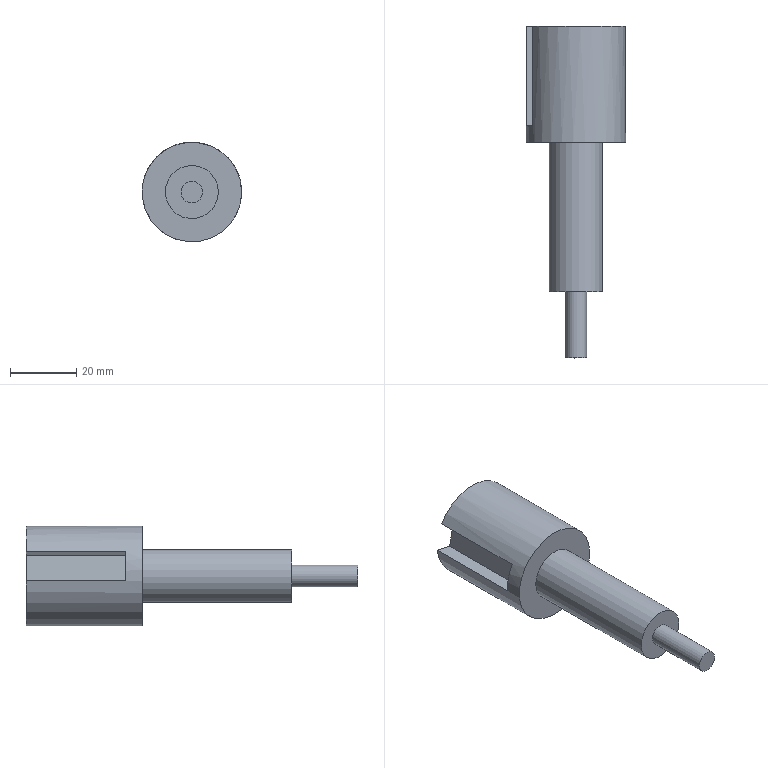Part | STEP file | SN10_006_001_PILOTO | 1 solid | 17 faces | box 30 x 100 x 30 mm | volume 30633 mm3 | plane 12 | cylinder 4 | cone 1 | commonest cylinder face diameters 6.5 x1 6.917 x1 16 x1 30 x1
STEP:
#1=CARTESIAN_POINT('',(0.,0.,0.));
#2=DIRECTION('',(0.,0.,1.));
#3=DIRECTION('',(1.,0.,0.));
#4=AXIS2_PLACEMENT_3D('',#1,#2,#3);
#5=CARTESIAN_POINT('',(381.092,-494.15,330.576));
#6=VERTEX_POINT('',#5);
#7=CARTESIAN_POINT('',(378.057,-494.15,328.918));
#8=DIRECTION('',(0.,1.,0.));
#9=DIRECTION('',(1.,0.,0.));
#10=AXIS2_PLACEMENT_3D('',#7,#8,#9);
#11=CIRCLE('',#10,3.458);
#12=CARTESIAN_POINT('',(378.057,-495.569,328.918));
#13=DIRECTION('',(0.,1.,0.));
#14=DIRECTION('',(0.8776,0.,0.4794));
#15=AXIS2_PLACEMENT_3D('',#12,#13,#14);
#16=CONICAL_SURFACE('',#15,1.,1.047);
#17=CARTESIAN_POINT('',(-5.783,1.419));
#18=DIRECTION('',(1.,0.));
#19=VECTOR('',#18,1.);
#20=LINE('',#17,#19);
#21=(GEOMETRIC_REPRESENTATION_CONTEXT(2)PARAMETRIC_REPRESENTATION_CONTEXT()REPRESENTATION_CONTEXT('',''));
#22=DEFINITIONAL_REPRESENTATION('',(#20),#21);
#23=PCURVE('',#16,#22);
#24=CARTESIAN_POINT('',(378.057,-476.25,328.918));
#25=DIRECTION('',(0.,-1.,0.));
#26=DIRECTION('',(0.8776,0.,0.4794));
#27=AXIS2_PLACEMENT_3D('',#24,#25,#26);
#28=CYLINDRICAL_SURFACE('',#27,3.458);
#29=CARTESIAN_POINT('',(12.066,17.9));
#30=DIRECTION('',(-1.,0.));
#31=VECTOR('',#30,1.);
#32=LINE('',#29,#31);
#33=(GEOMETRIC_REPRESENTATION_CONTEXT(2)PARAMETRIC_REPRESENTATION_CONTEXT()REPRESENTATION_CONTEXT('',''));
#34=DEFINITIONAL_REPRESENTATION('',(#32),#33);
#35=PCURVE('',#28,#34);
#36=SURFACE_CURVE('',#11,(#23,#35),.PCURVE_S1.);
#37=EDGE_CURVE('',#6,#6,#36,.T.);
#38=ORIENTED_EDGE('',*,*,#37,.F.);
#39=CARTESIAN_POINT('',(378.057,-496.147,328.918));
#40=VERTEX_POINT('',#39);
#41=CARTESIAN_POINT('',(378.057,-496.147,328.918));
#42=CARTESIAN_POINT('',(381.092,-494.15,330.576));
#43=B_SPLINE_CURVE_WITH_KNOTS('',1,(#41,#42),.UNSPECIFIED.,.F.,.F.,(2,2),(-1.155,2.839),.PIECEWISE_BEZIER_KNOTS.);
#44=CARTESIAN_POINT('',(0.,0.));
#45=DIRECTION('',(0.,1.));
#46=VECTOR('',#45,1.);
#47=LINE('',#44,#46);
#48=(GEOMETRIC_REPRESENTATION_CONTEXT(2)PARAMETRIC_REPRESENTATION_CONTEXT()REPRESENTATION_CONTEXT('',''));
#49=DEFINITIONAL_REPRESENTATION('',(#47),#48);
#50=PCURVE('',#16,#49);
#51=CARTESIAN_POINT('',(6.283,0.));
#52=DIRECTION('',(0.,1.));
#53=VECTOR('',#52,1.);
#54=LINE('',#51,#53);
#55=(GEOMETRIC_REPRESENTATION_CONTEXT(2)PARAMETRIC_REPRESENTATION_CONTEXT()REPRESENTATION_CONTEXT('',''));
#56=DEFINITIONAL_REPRESENTATION('',(#54),#55);
#57=PCURVE('',#16,#56);
#58=SEAM_CURVE('',#43,(#50,#57),.PCURVE_S1.);
#59=EDGE_CURVE('',#40,#6,#58,.T.);
#60=ORIENTED_EDGE('',*,*,#59,.F.);
#61=ORIENTED_EDGE('',*,*,#59,.T.);
#62=EDGE_LOOP('',(#38,#60,#61));
#63=FACE_BOUND('',#62,.F.);
#64=ADVANCED_FACE('',(#63),#16,.F.);
#65=CARTESIAN_POINT('',(391.135,-476.15,321.571));
#66=VERTEX_POINT('',#65);
#67=CARTESIAN_POINT('',(389.46,-476.15,319.173));
#68=VERTEX_POINT('',#67);
#69=CARTESIAN_POINT('',(378.057,-476.15,328.918));
#70=DIRECTION('',(0.,1.,0.));
#71=DIRECTION('',(1.,0.,0.));
#72=AXIS2_PLACEMENT_3D('',#69,#70,#71);
#73=CIRCLE('',#72,15.);
#74=CARTESIAN_POINT('',(392.736,-476.15,325.833));
#75=DIRECTION('',(0.,1.,0.));
#76=DIRECTION('',(0.,0.,1.));
#77=AXIS2_PLACEMENT_3D('',#74,#75,#76);
#78=PLANE('',#77);
#79=CARTESIAN_POINT('',(3.085,-14.679));
#80=DIRECTION('',(0.,1.));
#81=AXIS2_PLACEMENT_2D('',#79,#80);
#82=CIRCLE('',#81,15.);
#83=(GEOMETRIC_REPRESENTATION_CONTEXT(2)PARAMETRIC_REPRESENTATION_CONTEXT()REPRESENTATION_CONTEXT('',''));
#84=DEFINITIONAL_REPRESENTATION('',(#82),#83);
#85=PCURVE('',#78,#84);
#86=CARTESIAN_POINT('',(378.057,-526.15,328.918));
#87=DIRECTION('',(0.,1.,0.));
#88=DIRECTION('',(0.7602,0.,-0.6496));
#89=AXIS2_PLACEMENT_3D('',#86,#87,#88);
#90=CYLINDRICAL_SURFACE('',#89,15.);
#91=CARTESIAN_POINT('',(5.576,50.));
#92=DIRECTION('',(1.,0.));
#93=VECTOR('',#92,1.);
#94=LINE('',#91,#93);
#95=(GEOMETRIC_REPRESENTATION_CONTEXT(2)PARAMETRIC_REPRESENTATION_CONTEXT()REPRESENTATION_CONTEXT('',''));
#96=DEFINITIONAL_REPRESENTATION('',(#94),#95);
#97=PCURVE('',#90,#96);
#98=SURFACE_CURVE('',#73,(#85,#97),.PCURVE_S1.);
#99=EDGE_CURVE('',#66,#68,#98,.T.);
#100=ORIENTED_EDGE('',*,*,#99,.T.);
#101=CARTESIAN_POINT('',(363.128,-476.15,327.457));
#102=VERTEX_POINT('',#101);
#103=CARTESIAN_POINT('',(378.057,-476.15,328.918));
#104=DIRECTION('',(0.,1.,0.));
#105=DIRECTION('',(1.,0.,0.));
#106=AXIS2_PLACEMENT_3D('',#103,#104,#105);
#107=CIRCLE('',#106,15.);
#108=CARTESIAN_POINT('',(3.085,-14.679));
#109=DIRECTION('',(0.,1.));
#110=AXIS2_PLACEMENT_2D('',#108,#109);
#111=CIRCLE('',#110,15.);
#112=(GEOMETRIC_REPRESENTATION_CONTEXT(2)PARAMETRIC_REPRESENTATION_CONTEXT()REPRESENTATION_CONTEXT('',''));
#113=DEFINITIONAL_REPRESENTATION('',(#111),#112);
#114=PCURVE('',#78,#113);
#115=CARTESIAN_POINT('',(-0.7071,50.));
#116=DIRECTION('',(1.,0.));
#117=VECTOR('',#116,1.);
#118=LINE('',#115,#117);
#119=(GEOMETRIC_REPRESENTATION_CONTEXT(2)PARAMETRIC_REPRESENTATION_CONTEXT()REPRESENTATION_CONTEXT('',''));
#120=DEFINITIONAL_REPRESENTATION('',(#118),#119);
#121=PCURVE('',#90,#120);
#122=SURFACE_CURVE('',#107,(#114,#121),.PCURVE_S1.);
#123=EDGE_CURVE('',#68,#102,#122,.T.);
#124=ORIENTED_EDGE('',*,*,#123,.T.);
#125=CARTESIAN_POINT('',(368.324,-476.15,326.365));
#126=VERTEX_POINT('',#125);
#127=CARTESIAN_POINT('',(363.128,-476.15,327.457));
#128=DIRECTION('',(0.9786,0.,-0.2056));
#129=VECTOR('',#128,1.);
#130=LINE('',#127,#129);
#131=CARTESIAN_POINT('',(1.623,-29.608));
#132=DIRECTION('',(-0.2056,0.9786));
#133=VECTOR('',#132,1.);
#134=LINE('',#131,#133);
#135=(GEOMETRIC_REPRESENTATION_CONTEXT(2)PARAMETRIC_REPRESENTATION_CONTEXT()REPRESENTATION_CONTEXT('',''));
#136=DEFINITIONAL_REPRESENTATION('',(#134),#135);
#137=PCURVE('',#78,#136);
#138=CARTESIAN_POINT('',(363.128,-476.15,327.457));
#139=DIRECTION('',(-0.2056,0.,-0.9786));
#140=DIRECTION('',(-0.9786,0.,0.2056));
#141=AXIS2_PLACEMENT_3D('',#138,#139,#140);
#142=PLANE('',#141);
#143=CARTESIAN_POINT('',(0.,0.));
#144=DIRECTION('',(-1.,0.));
#145=VECTOR('',#144,1.);
#146=LINE('',#143,#145);
#147=(GEOMETRIC_REPRESENTATION_CONTEXT(2)PARAMETRIC_REPRESENTATION_CONTEXT()REPRESENTATION_CONTEXT('',''));
#148=DEFINITIONAL_REPRESENTATION('',(#146),#147);
#149=PCURVE('',#142,#148);
#150=SURFACE_CURVE('',#130,(#137,#149),.PCURVE_S1.);
#151=EDGE_CURVE('',#102,#126,#150,.T.);
#152=ORIENTED_EDGE('',*,*,#151,.T.);
#153=CARTESIAN_POINT('',(370.175,-476.15,335.172));
#154=VERTEX_POINT('',#153);
#155=CARTESIAN_POINT('',(368.324,-476.15,326.365));
#156=DIRECTION('',(0.2056,0.,0.9786));
#157=VECTOR('',#156,1.);
#158=LINE('',#155,#157);
#159=CARTESIAN_POINT('',(0.5316,-24.412));
#160=DIRECTION('',(0.9786,0.2056));
#161=VECTOR('',#160,1.);
#162=LINE('',#159,#161);
#163=(GEOMETRIC_REPRESENTATION_CONTEXT(2)PARAMETRIC_REPRESENTATION_CONTEXT()REPRESENTATION_CONTEXT('',''));
#164=DEFINITIONAL_REPRESENTATION('',(#162),#163);
#165=PCURVE('',#78,#164);
#166=CARTESIAN_POINT('',(368.324,-476.15,326.365));
#167=DIRECTION('',(0.9786,0.,-0.2056));
#168=DIRECTION('',(-0.2056,0.,-0.9786));
#169=AXIS2_PLACEMENT_3D('',#166,#167,#168);
#170=PLANE('',#169);
#171=CARTESIAN_POINT('',(0.,0.));
#172=DIRECTION('',(-1.,0.));
#173=VECTOR('',#172,1.);
#174=LINE('',#171,#173);
#175=(GEOMETRIC_REPRESENTATION_CONTEXT(2)PARAMETRIC_REPRESENTATION_CONTEXT()REPRESENTATION_CONTEXT('',''));
#176=DEFINITIONAL_REPRESENTATION('',(#174),#175);
#177=PCURVE('',#170,#176);
#178=SURFACE_CURVE('',#158,(#165,#177),.PCURVE_S1.);
#179=EDGE_CURVE('',#126,#154,#178,.T.);
#180=ORIENTED_EDGE('',*,*,#179,.T.);
#181=CARTESIAN_POINT('',(364.979,-476.15,336.264));
#182=VERTEX_POINT('',#181);
#183=CARTESIAN_POINT('',(370.175,-476.15,335.172));
#184=DIRECTION('',(-0.9786,0.,0.2056));
#185=VECTOR('',#184,1.);
#186=LINE('',#183,#185);
#187=CARTESIAN_POINT('',(9.339,-22.562));
#188=DIRECTION('',(0.2056,-0.9786));
#189=VECTOR('',#188,1.);
#190=LINE('',#187,#189);
#191=(GEOMETRIC_REPRESENTATION_CONTEXT(2)PARAMETRIC_REPRESENTATION_CONTEXT()REPRESENTATION_CONTEXT('',''));
#192=DEFINITIONAL_REPRESENTATION('',(#190),#191);
#193=PCURVE('',#78,#192);
#194=CARTESIAN_POINT('',(370.175,-476.15,335.172));
#195=DIRECTION('',(0.2056,0.,0.9786));
#196=DIRECTION('',(0.9786,0.,-0.2056));
#197=AXIS2_PLACEMENT_3D('',#194,#195,#196);
#198=PLANE('',#197);
#199=CARTESIAN_POINT('',(0.000000001,0.));
#200=DIRECTION('',(-1.,0.));
#201=VECTOR('',#200,1.);
#202=LINE('',#199,#201);
#203=(GEOMETRIC_REPRESENTATION_CONTEXT(2)PARAMETRIC_REPRESENTATION_CONTEXT()REPRESENTATION_CONTEXT('',''));
#204=DEFINITIONAL_REPRESENTATION('',(#202),#203);
#205=PCURVE('',#198,#204);
#206=SURFACE_CURVE('',#186,(#193,#205),.PCURVE_S1.);
#207=EDGE_CURVE('',#154,#182,#206,.T.);
#208=ORIENTED_EDGE('',*,*,#207,.T.);
#209=CARTESIAN_POINT('',(392.985,-476.15,330.379));
#210=VERTEX_POINT('',#209);
#211=CARTESIAN_POINT('',(378.057,-476.15,328.918));
#212=DIRECTION('',(0.,1.,0.));
#213=DIRECTION('',(1.,0.,0.));
#214=AXIS2_PLACEMENT_3D('',#211,#212,#213);
#215=CIRCLE('',#214,15.);
#216=CARTESIAN_POINT('',(3.085,-14.679));
#217=DIRECTION('',(0.,1.));
#218=AXIS2_PLACEMENT_2D('',#216,#217);
#219=CIRCLE('',#218,15.);
#220=(GEOMETRIC_REPRESENTATION_CONTEXT(2)PARAMETRIC_REPRESENTATION_CONTEXT()REPRESENTATION_CONTEXT('',''));
#221=DEFINITIONAL_REPRESENTATION('',(#219),#220);
#222=PCURVE('',#78,#221);
#223=CARTESIAN_POINT('',(-0.7071,50.));
#224=DIRECTION('',(1.,0.));
#225=VECTOR('',#224,1.);
#226=LINE('',#223,#225);
#227=(GEOMETRIC_REPRESENTATION_CONTEXT(2)PARAMETRIC_REPRESENTATION_CONTEXT()REPRESENTATION_CONTEXT('',''));
#228=DEFINITIONAL_REPRESENTATION('',(#226),#227);
#229=PCURVE('',#90,#228);
#230=SURFACE_CURVE('',#215,(#222,#229),.PCURVE_S1.);
#231=EDGE_CURVE('',#182,#210,#230,.T.);
#232=ORIENTED_EDGE('',*,*,#231,.T.);
#233=CARTESIAN_POINT('',(387.79,-476.15,331.471));
#234=VERTEX_POINT('',#233);
#235=CARTESIAN_POINT('',(392.985,-476.15,330.379));
#236=DIRECTION('',(-0.9786,0.,0.2056));
#237=VECTOR('',#236,1.);
#238=LINE('',#235,#237);
#239=CARTESIAN_POINT('',(4.546,0.2492));
#240=DIRECTION('',(0.2056,-0.9786));
#241=VECTOR('',#240,1.);
#242=LINE('',#239,#241);
#243=(GEOMETRIC_REPRESENTATION_CONTEXT(2)PARAMETRIC_REPRESENTATION_CONTEXT()REPRESENTATION_CONTEXT('',''));
#244=DEFINITIONAL_REPRESENTATION('',(#242),#243);
#245=PCURVE('',#78,#244);
#246=CARTESIAN_POINT('',(370.175,-476.15,335.172));
#247=DIRECTION('',(0.2056,0.,0.9786));
#248=DIRECTION('',(0.9786,0.,-0.2056));
#249=AXIS2_PLACEMENT_3D('',#246,#247,#248);
#250=PLANE('',#249);
#251=CARTESIAN_POINT('',(23.309,0.));
#252=DIRECTION('',(-1.,0.));
#253=VECTOR('',#252,1.);
#254=LINE('',#251,#253);
#255=(GEOMETRIC_REPRESENTATION_CONTEXT(2)PARAMETRIC_REPRESENTATION_CONTEXT()REPRESENTATION_CONTEXT('',''));
#256=DEFINITIONAL_REPRESENTATION('',(#254),#255);
#257=PCURVE('',#250,#256);
#258=SURFACE_CURVE('',#238,(#245,#257),.PCURVE_S1.);
#259=EDGE_CURVE('',#210,#234,#258,.T.);
#260=ORIENTED_EDGE('',*,*,#259,.T.);
#261=CARTESIAN_POINT('',(385.939,-476.15,322.663));
#262=VERTEX_POINT('',#261);
#263=CARTESIAN_POINT('',(385.939,-476.15,322.663));
#264=DIRECTION('',(0.2056,0.,0.9786));
#265=VECTOR('',#264,1.);
#266=LINE('',#263,#265);
#267=CARTESIAN_POINT('',(-3.17,-6.797));
#268=DIRECTION('',(0.9786,0.2056));
#269=VECTOR('',#268,1.);
#270=LINE('',#267,#269);
#271=(GEOMETRIC_REPRESENTATION_CONTEXT(2)PARAMETRIC_REPRESENTATION_CONTEXT()REPRESENTATION_CONTEXT('',''));
#272=DEFINITIONAL_REPRESENTATION('',(#270),#271);
#273=PCURVE('',#78,#272);
#274=CARTESIAN_POINT('',(385.939,-476.15,322.663));
#275=DIRECTION('',(0.9786,0.,-0.2056));
#276=DIRECTION('',(-0.2056,0.,-0.9786));
#277=AXIS2_PLACEMENT_3D('',#274,#275,#276);
#278=PLANE('',#277);
#279=CARTESIAN_POINT('',(0.,0.));
#280=DIRECTION('',(-1.,0.));
#281=VECTOR('',#280,1.);
#282=LINE('',#279,#281);
#283=(GEOMETRIC_REPRESENTATION_CONTEXT(2)PARAMETRIC_REPRESENTATION_CONTEXT()REPRESENTATION_CONTEXT('',''));
#284=DEFINITIONAL_REPRESENTATION('',(#282),#283);
#285=PCURVE('',#278,#284);
#286=SURFACE_CURVE('',#266,(#273,#285),.PCURVE_S1.);
#287=EDGE_CURVE('',#262,#234,#286,.T.);
#288=ORIENTED_EDGE('',*,*,#287,.F.);
#289=CARTESIAN_POINT('',(385.939,-476.15,322.663));
#290=DIRECTION('',(0.9786,0.,-0.2056));
#291=VECTOR('',#290,1.);
#292=LINE('',#289,#291);
#293=CARTESIAN_POINT('',(-3.17,-6.797));
#294=DIRECTION('',(-0.2056,0.9786));
#295=VECTOR('',#294,1.);
#296=LINE('',#293,#295);
#297=(GEOMETRIC_REPRESENTATION_CONTEXT(2)PARAMETRIC_REPRESENTATION_CONTEXT()REPRESENTATION_CONTEXT('',''));
#298=DEFINITIONAL_REPRESENTATION('',(#296),#297);
#299=PCURVE('',#78,#298);
#300=CARTESIAN_POINT('',(363.128,-476.15,327.457));
#301=DIRECTION('',(-0.2056,0.,-0.9786));
#302=DIRECTION('',(-0.9786,0.,0.2056));
#303=AXIS2_PLACEMENT_3D('',#300,#301,#302);
#304=PLANE('',#303);
#305=CARTESIAN_POINT('',(-23.309,0.));
#306=DIRECTION('',(-1.,0.));
#307=VECTOR('',#306,1.);
#308=LINE('',#305,#307);
#309=(GEOMETRIC_REPRESENTATION_CONTEXT(2)PARAMETRIC_REPRESENTATION_CONTEXT()REPRESENTATION_CONTEXT('',''));
#310=DEFINITIONAL_REPRESENTATION('',(#308),#309);
#311=PCURVE('',#304,#310);
#312=SURFACE_CURVE('',#292,(#299,#311),.PCURVE_S1.);
#313=EDGE_CURVE('',#262,#66,#312,.T.);
#314=ORIENTED_EDGE('',*,*,#313,.T.);
#315=EDGE_LOOP('',(#100,#124,#152,#180,#208,#232,#260,#288,#314));
#316=FACE_BOUND('',#315,.T.);
#317=CARTESIAN_POINT('',(381.092,-476.15,330.576));
#318=VERTEX_POINT('',#317);
#319=CARTESIAN_POINT('',(378.057,-476.15,328.918));
#320=DIRECTION('',(0.,1.,0.));
#321=DIRECTION('',(1.,0.,0.));
#322=AXIS2_PLACEMENT_3D('',#319,#320,#321);
#323=CIRCLE('',#322,3.458);
#324=CARTESIAN_POINT('',(3.085,-14.679));
#325=DIRECTION('',(0.,1.));
#326=AXIS2_PLACEMENT_2D('',#324,#325);
#327=CIRCLE('',#326,3.458);
#328=(GEOMETRIC_REPRESENTATION_CONTEXT(2)PARAMETRIC_REPRESENTATION_CONTEXT()REPRESENTATION_CONTEXT('',''));
#329=DEFINITIONAL_REPRESENTATION('',(#327),#328);
#330=PCURVE('',#78,#329);
#331=CARTESIAN_POINT('',(12.066,-0.1));
#332=DIRECTION('',(-1.,0.));
#333=VECTOR('',#332,1.);
#334=LINE('',#331,#333);
#335=(GEOMETRIC_REPRESENTATION_CONTEXT(2)PARAMETRIC_REPRESENTATION_CONTEXT()REPRESENTATION_CONTEXT('',''));
#336=DEFINITIONAL_REPRESENTATION('',(#334),#335);
#337=PCURVE('',#28,#336);
#338=SURFACE_CURVE('',#323,(#330,#337),.PCURVE_S1.);
#339=EDGE_CURVE('',#318,#318,#338,.T.);
#340=ORIENTED_EDGE('',*,*,#339,.F.);
#341=EDGE_LOOP('',(#340));
#342=FACE_BOUND('',#341,.T.);
#343=ADVANCED_FACE('',(#316,#342),#78,.T.);
#344=ORIENTED_EDGE('',*,*,#123,.F.);
#345=CARTESIAN_POINT('',(389.46,-511.15,319.173));
#346=VERTEX_POINT('',#345);
#347=CARTESIAN_POINT('',(389.46,-511.15,319.173));
#348=CARTESIAN_POINT('',(389.46,-476.15,319.173));
#349=B_SPLINE_CURVE_WITH_KNOTS('',1,(#347,#348),.UNSPECIFIED.,.F.,.F.,(2,2),(15.,50.),.PIECEWISE_BEZIER_KNOTS.);
#350=CARTESIAN_POINT('',(0.,0.));
#351=DIRECTION('',(0.,1.));
#352=VECTOR('',#351,1.);
#353=LINE('',#350,#352);
#354=(GEOMETRIC_REPRESENTATION_CONTEXT(2)PARAMETRIC_REPRESENTATION_CONTEXT()REPRESENTATION_CONTEXT('',''));
#355=DEFINITIONAL_REPRESENTATION('',(#353),#354);
#356=PCURVE('',#90,#355);
#357=CARTESIAN_POINT('',(6.283,0.));
#358=DIRECTION('',(0.,1.));
#359=VECTOR('',#358,1.);
#360=LINE('',#357,#359);
#361=(GEOMETRIC_REPRESENTATION_CONTEXT(2)PARAMETRIC_REPRESENTATION_CONTEXT()REPRESENTATION_CONTEXT('',''));
#362=DEFINITIONAL_REPRESENTATION('',(#360),#361);
#363=PCURVE('',#90,#362);
#364=SEAM_CURVE('',#349,(#356,#363),.PCURVE_S1.);
#365=EDGE_CURVE('',#346,#68,#364,.T.);
#366=ORIENTED_EDGE('',*,*,#365,.F.);
#367=CARTESIAN_POINT('',(378.057,-511.15,328.918));
#368=DIRECTION('',(0.,1.,0.));
#369=DIRECTION('',(1.,0.,0.));
#370=AXIS2_PLACEMENT_3D('',#367,#368,#369);
#371=CIRCLE('',#370,15.);
#372=CARTESIAN_POINT('',(-0.7071,15.));
#373=DIRECTION('',(1.,0.));
#374=VECTOR('',#373,1.);
#375=LINE('',#372,#374);
#376=(GEOMETRIC_REPRESENTATION_CONTEXT(2)PARAMETRIC_REPRESENTATION_CONTEXT()REPRESENTATION_CONTEXT('',''));
#377=DEFINITIONAL_REPRESENTATION('',(#375),#376);
#378=PCURVE('',#90,#377);
#379=CARTESIAN_POINT('',(385.886,-511.15,327.273));
#380=DIRECTION('',(0.,1.,0.));
#381=DIRECTION('',(0.,0.,1.));
#382=AXIS2_PLACEMENT_3D('',#379,#380,#381);
#383=PLANE('',#382);
#384=CARTESIAN_POINT('',(1.645,-7.829));
#385=DIRECTION('',(0.,1.));
#386=AXIS2_PLACEMENT_2D('',#384,#385);
#387=CIRCLE('',#386,15.);
#388=(GEOMETRIC_REPRESENTATION_CONTEXT(2)PARAMETRIC_REPRESENTATION_CONTEXT()REPRESENTATION_CONTEXT('',''));
#389=DEFINITIONAL_REPRESENTATION('',(#387),#388);
#390=PCURVE('',#383,#389);
#391=SURFACE_CURVE('',#371,(#378,#390),.PCURVE_S1.);
#392=EDGE_CURVE('',#346,#346,#391,.T.);
#393=ORIENTED_EDGE('',*,*,#392,.T.);
#394=ORIENTED_EDGE('',*,*,#365,.T.);
#395=ORIENTED_EDGE('',*,*,#99,.F.);
#396=CARTESIAN_POINT('',(391.135,-506.15,321.571));
#397=VERTEX_POINT('',#396);
#398=CARTESIAN_POINT('',(391.135,-506.15,321.571));
#399=DIRECTION('',(0.,1.,0.));
#400=VECTOR('',#399,1.);
#401=LINE('',#398,#400);
#402=CARTESIAN_POINT('',(6.088,20.));
#403=DIRECTION('',(0.,1.));
#404=VECTOR('',#403,1.);
#405=LINE('',#402,#404);
#406=(GEOMETRIC_REPRESENTATION_CONTEXT(2)PARAMETRIC_REPRESENTATION_CONTEXT()REPRESENTATION_CONTEXT('',''));
#407=DEFINITIONAL_REPRESENTATION('',(#405),#406);
#408=PCURVE('',#90,#407);
#409=CARTESIAN_POINT('',(-28.618,-30.));
#410=DIRECTION('',(0.,1.));
#411=VECTOR('',#410,1.);
#412=LINE('',#409,#411);
#413=(GEOMETRIC_REPRESENTATION_CONTEXT(2)PARAMETRIC_REPRESENTATION_CONTEXT()REPRESENTATION_CONTEXT('',''));
#414=DEFINITIONAL_REPRESENTATION('',(#412),#413);
#415=PCURVE('',#304,#414);
#416=SURFACE_CURVE('',#401,(#408,#415),.PCURVE_S1.);
#417=EDGE_CURVE('',#397,#66,#416,.T.);
#418=ORIENTED_EDGE('',*,*,#417,.F.);
#419=CARTESIAN_POINT('',(392.985,-506.15,330.379));
#420=VERTEX_POINT('',#419);
#421=CARTESIAN_POINT('',(378.057,-506.15,328.918));
#422=DIRECTION('',(0.,1.,0.));
#423=DIRECTION('',(1.,0.,0.));
#424=AXIS2_PLACEMENT_3D('',#421,#422,#423);
#425=CIRCLE('',#424,15.);
#426=CARTESIAN_POINT('',(-0.7071,20.));
#427=DIRECTION('',(1.,0.));
#428=VECTOR('',#427,1.);
#429=LINE('',#426,#428);
#430=(GEOMETRIC_REPRESENTATION_CONTEXT(2)PARAMETRIC_REPRESENTATION_CONTEXT()REPRESENTATION_CONTEXT('',''));
#431=DEFINITIONAL_REPRESENTATION('',(#429),#430);
#432=PCURVE('',#90,#431);
#433=CARTESIAN_POINT('',(0.,-506.15,0.));
#434=DIRECTION('',(0.,1.,0.));
#435=DIRECTION('',(0.,0.,1.));
#436=AXIS2_PLACEMENT_3D('',#433,#434,#435);
#437=PLANE('',#436);
#438=CARTESIAN_POINT('',(328.918,378.057));
#439=DIRECTION('',(0.,1.));
#440=AXIS2_PLACEMENT_2D('',#438,#439);
#441=CIRCLE('',#440,15.);
#442=(GEOMETRIC_REPRESENTATION_CONTEXT(2)PARAMETRIC_REPRESENTATION_CONTEXT()REPRESENTATION_CONTEXT('',''));
#443=DEFINITIONAL_REPRESENTATION('',(#441),#442);
#444=PCURVE('',#437,#443);
#445=SURFACE_CURVE('',#425,(#432,#444),.PCURVE_S1.);
#446=EDGE_CURVE('',#420,#397,#445,.T.);
#447=ORIENTED_EDGE('',*,*,#446,.F.);
#448=CARTESIAN_POINT('',(392.985,-506.15,330.379));
#449=DIRECTION('',(0.,1.,0.));
#450=VECTOR('',#449,1.);
#451=LINE('',#448,#450);
#452=CARTESIAN_POINT('',(5.478,20.));
#453=DIRECTION('',(0.,1.));
#454=VECTOR('',#453,1.);
#455=LINE('',#452,#454);
#456=(GEOMETRIC_REPRESENTATION_CONTEXT(2)PARAMETRIC_REPRESENTATION_CONTEXT()REPRESENTATION_CONTEXT('',''));
#457=DEFINITIONAL_REPRESENTATION('',(#455),#456);
#458=PCURVE('',#90,#457);
#459=CARTESIAN_POINT('',(23.309,-30.));
#460=DIRECTION('',(0.,1.));
#461=VECTOR('',#460,1.);
#462=LINE('',#459,#461);
#463=(GEOMETRIC_REPRESENTATION_CONTEXT(2)PARAMETRIC_REPRESENTATION_CONTEXT()REPRESENTATION_CONTEXT('',''));
#464=DEFINITIONAL_REPRESENTATION('',(#462),#463);
#465=PCURVE('',#250,#464);
#466=SURFACE_CURVE('',#451,(#458,#465),.PCURVE_S1.);
#467=EDGE_CURVE('',#420,#210,#466,.T.);
#468=ORIENTED_EDGE('',*,*,#467,.T.);
#469=ORIENTED_EDGE('',*,*,#231,.F.);
#470=CARTESIAN_POINT('',(364.979,-506.15,336.264));
#471=VERTEX_POINT('',#470);
#472=CARTESIAN_POINT('',(364.979,-506.15,336.264));
#473=DIRECTION('',(0.,1.,0.));
#474=VECTOR('',#473,1.);
#475=LINE('',#472,#474);
#476=CARTESIAN_POINT('',(2.946,20.));
#477=DIRECTION('',(0.,1.));
#478=VECTOR('',#477,1.);
#479=LINE('',#476,#478);
#480=(GEOMETRIC_REPRESENTATION_CONTEXT(2)PARAMETRIC_REPRESENTATION_CONTEXT()REPRESENTATION_CONTEXT('',''));
#481=DEFINITIONAL_REPRESENTATION('',(#479),#480);
#482=PCURVE('',#90,#481);
#483=CARTESIAN_POINT('',(-5.309,-30.));
#484=DIRECTION('',(0.,1.));
#485=VECTOR('',#484,1.);
#486=LINE('',#483,#485);
#487=(GEOMETRIC_REPRESENTATION_CONTEXT(2)PARAMETRIC_REPRESENTATION_CONTEXT()REPRESENTATION_CONTEXT('',''));
#488=DEFINITIONAL_REPRESENTATION('',(#486),#487);
#489=PCURVE('',#198,#488);
#490=SURFACE_CURVE('',#475,(#482,#489),.PCURVE_S1.);
#491=EDGE_CURVE('',#471,#182,#490,.T.);
#492=ORIENTED_EDGE('',*,*,#491,.F.);
#493=CARTESIAN_POINT('',(363.128,-506.15,327.457));
#494=VERTEX_POINT('',#493);
#495=CARTESIAN_POINT('',(378.057,-506.15,328.918));
#496=DIRECTION('',(0.,1.,0.));
#497=DIRECTION('',(1.,0.,0.));
#498=AXIS2_PLACEMENT_3D('',#495,#496,#497);
#499=CIRCLE('',#498,15.);
#500=CARTESIAN_POINT('',(-0.7071,20.));
#501=DIRECTION('',(1.,0.));
#502=VECTOR('',#501,1.);
#503=LINE('',#500,#502);
#504=(GEOMETRIC_REPRESENTATION_CONTEXT(2)PARAMETRIC_REPRESENTATION_CONTEXT()REPRESENTATION_CONTEXT('',''));
#505=DEFINITIONAL_REPRESENTATION('',(#503),#504);
#506=PCURVE('',#90,#505);
#507=CARTESIAN_POINT('',(0.,-506.15,0.));
#508=DIRECTION('',(0.,1.,0.));
#509=DIRECTION('',(0.,0.,1.));
#510=AXIS2_PLACEMENT_3D('',#507,#508,#509);
#511=PLANE('',#510);
#512=CARTESIAN_POINT('',(328.918,378.057));
#513=DIRECTION('',(0.,1.));
#514=AXIS2_PLACEMENT_2D('',#512,#513);
#515=CIRCLE('',#514,15.);
#516=(GEOMETRIC_REPRESENTATION_CONTEXT(2)PARAMETRIC_REPRESENTATION_CONTEXT()REPRESENTATION_CONTEXT('',''));
#517=DEFINITIONAL_REPRESENTATION('',(#515),#516);
#518=PCURVE('',#511,#517);
#519=SURFACE_CURVE('',#499,(#506,#518),.PCURVE_S1.);
#520=EDGE_CURVE('',#494,#471,#519,.T.);
#521=ORIENTED_EDGE('',*,*,#520,.F.);
#522=CARTESIAN_POINT('',(363.128,-506.15,327.457));
#523=DIRECTION('',(0.,1.,0.));
#524=VECTOR('',#523,1.);
#525=LINE('',#522,#524);
#526=CARTESIAN_POINT('',(2.337,20.));
#527=DIRECTION('',(0.,1.));
#528=VECTOR('',#527,1.);
#529=LINE('',#526,#528);
#530=(GEOMETRIC_REPRESENTATION_CONTEXT(2)PARAMETRIC_REPRESENTATION_CONTEXT()REPRESENTATION_CONTEXT('',''));
#531=DEFINITIONAL_REPRESENTATION('',(#529),#530);
#532=PCURVE('',#90,#531);
#533=CARTESIAN_POINT('',(0.,-30.));
#534=DIRECTION('',(0.,1.));
#535=VECTOR('',#534,1.);
#536=LINE('',#533,#535);
#537=(GEOMETRIC_REPRESENTATION_CONTEXT(2)PARAMETRIC_REPRESENTATION_CONTEXT()REPRESENTATION_CONTEXT('',''));
#538=DEFINITIONAL_REPRESENTATION('',(#536),#537);
#539=PCURVE('',#142,#538);
#540=SURFACE_CURVE('',#525,(#532,#539),.PCURVE_S1.);
#541=EDGE_CURVE('',#494,#102,#540,.T.);
#542=ORIENTED_EDGE('',*,*,#541,.T.);
#543=EDGE_LOOP('',(#344,#366,#393,#394,#395,#418,#447,#468,#469,#492,#521,#542));
#544=FACE_BOUND('',#543,.T.);
#545=ADVANCED_FACE('',(#544),#90,.T.);
#546=ORIENTED_EDGE('',*,*,#392,.F.);
#547=EDGE_LOOP('',(#546));
#548=FACE_BOUND('',#547,.T.);
#549=CARTESIAN_POINT('',(384.139,-511.15,323.721));
#550=VERTEX_POINT('',#549);
#551=CARTESIAN_POINT('',(378.057,-511.15,328.918));
#552=DIRECTION('',(0.,1.,0.));
#553=DIRECTION('',(1.,0.,0.));
#554=AXIS2_PLACEMENT_3D('',#551,#552,#553);
#555=CIRCLE('',#554,8.);
#556=CARTESIAN_POINT('',(1.645,-7.829));
#557=DIRECTION('',(0.,1.));
#558=AXIS2_PLACEMENT_2D('',#556,#557);
#559=CIRCLE('',#558,8.);
#560=(GEOMETRIC_REPRESENTATION_CONTEXT(2)PARAMETRIC_REPRESENTATION_CONTEXT()REPRESENTATION_CONTEXT('',''));
#561=DEFINITIONAL_REPRESENTATION('',(#559),#560);
#562=PCURVE('',#383,#561);
#563=CARTESIAN_POINT('',(378.057,-526.15,328.918));
#564=DIRECTION('',(0.,1.,0.));
#565=DIRECTION('',(0.7602,0.,-0.6496));
#566=AXIS2_PLACEMENT_3D('',#563,#564,#565);
#567=CYLINDRICAL_SURFACE('',#566,8.);
#568=CARTESIAN_POINT('',(-0.7071,15.));
#569=DIRECTION('',(1.,0.));
#570=VECTOR('',#569,1.);
#571=LINE('',#568,#570);
#572=(GEOMETRIC_REPRESENTATION_CONTEXT(2)PARAMETRIC_REPRESENTATION_CONTEXT()REPRESENTATION_CONTEXT('',''));
#573=DEFINITIONAL_REPRESENTATION('',(#571),#572);
#574=PCURVE('',#567,#573);
#575=SURFACE_CURVE('',#555,(#562,#574),.PCURVE_S1.);
#576=EDGE_CURVE('',#550,#550,#575,.T.);
#577=ORIENTED_EDGE('',*,*,#576,.T.);
#578=EDGE_LOOP('',(#577));
#579=FACE_BOUND('',#578,.T.);
#580=ADVANCED_FACE('',(#548,#579),#383,.F.);
#581=CARTESIAN_POINT('',(384.139,-556.15,323.721));
#582=VERTEX_POINT('',#581);
#583=CARTESIAN_POINT('',(378.057,-556.15,328.918));
#584=DIRECTION('',(0.,1.,0.));
#585=DIRECTION('',(1.,0.,0.));
#586=AXIS2_PLACEMENT_3D('',#583,#584,#585);
#587=CIRCLE('',#586,8.);
#588=CARTESIAN_POINT('',(-0.7071,-30.));
#589=DIRECTION('',(1.,0.));
#590=VECTOR('',#589,1.);
#591=LINE('',#588,#590);
#592=(GEOMETRIC_REPRESENTATION_CONTEXT(2)PARAMETRIC_REPRESENTATION_CONTEXT()REPRESENTATION_CONTEXT('',''));
#593=DEFINITIONAL_REPRESENTATION('',(#591),#592);
#594=PCURVE('',#567,#593);
#595=CARTESIAN_POINT('',(381.237,-556.15,328.25));
#596=DIRECTION('',(0.,1.,0.));
#597=DIRECTION('',(0.,0.,1.));
#598=AXIS2_PLACEMENT_3D('',#595,#596,#597);
#599=PLANE('',#598);
#600=CARTESIAN_POINT('',(0.6683,-3.181));
#601=DIRECTION('',(0.,1.));
#602=AXIS2_PLACEMENT_2D('',#600,#601);
#603=CIRCLE('',#602,8.);
#604=(GEOMETRIC_REPRESENTATION_CONTEXT(2)PARAMETRIC_REPRESENTATION_CONTEXT()REPRESENTATION_CONTEXT('',''));
#605=DEFINITIONAL_REPRESENTATION('',(#603),#604);
#606=PCURVE('',#599,#605);
#607=SURFACE_CURVE('',#587,(#594,#606),.PCURVE_S1.);
#608=EDGE_CURVE('',#582,#582,#607,.T.);
#609=ORIENTED_EDGE('',*,*,#608,.T.);
#610=CARTESIAN_POINT('',(384.139,-556.15,323.721));
#611=CARTESIAN_POINT('',(384.139,-511.15,323.721));
#612=B_SPLINE_CURVE_WITH_KNOTS('',1,(#610,#611),.UNSPECIFIED.,.F.,.F.,(2,2),(-30.,15.),.PIECEWISE_BEZIER_KNOTS.);
#613=CARTESIAN_POINT('',(6.283,0.));
#614=DIRECTION('',(0.,1.));
#615=VECTOR('',#614,1.);
#616=LINE('',#613,#615);
#617=(GEOMETRIC_REPRESENTATION_CONTEXT(2)PARAMETRIC_REPRESENTATION_CONTEXT()REPRESENTATION_CONTEXT('',''));
#618=DEFINITIONAL_REPRESENTATION('',(#616),#617);
#619=PCURVE('',#567,#618);
#620=CARTESIAN_POINT('',(0.,0.));
#621=DIRECTION('',(0.,1.));
#622=VECTOR('',#621,1.);
#623=LINE('',#620,#622);
#624=(GEOMETRIC_REPRESENTATION_CONTEXT(2)PARAMETRIC_REPRESENTATION_CONTEXT()REPRESENTATION_CONTEXT('',''));
#625=DEFINITIONAL_REPRESENTATION('',(#623),#624);
#626=PCURVE('',#567,#625);
#627=SEAM_CURVE('',#612,(#619,#626),.PCURVE_S1.);
#628=EDGE_CURVE('',#582,#550,#627,.T.);
#629=ORIENTED_EDGE('',*,*,#628,.T.);
#630=ORIENTED_EDGE('',*,*,#576,.F.);
#631=ORIENTED_EDGE('',*,*,#628,.F.);
#632=EDGE_LOOP('',(#609,#629,#630,#631));
#633=FACE_BOUND('',#632,.T.);
#634=ADVANCED_FACE('',(#633),#567,.T.);
#635=ORIENTED_EDGE('',*,*,#608,.F.);
#636=EDGE_LOOP('',(#635));
#637=FACE_BOUND('',#636,.T.);
#638=CARTESIAN_POINT('',(380.528,-556.15,326.806));
#639=VERTEX_POINT('',#638);
#640=CARTESIAN_POINT('',(378.057,-556.15,328.918));
#641=DIRECTION('',(0.,1.,0.));
#642=DIRECTION('',(1.,0.,0.));
#643=AXIS2_PLACEMENT_3D('',#640,#641,#642);
#644=CIRCLE('',#643,3.25);
#645=CARTESIAN_POINT('',(0.6683,-3.181));
#646=DIRECTION('',(0.,1.));
#647=AXIS2_PLACEMENT_2D('',#645,#646);
#648=CIRCLE('',#647,3.25);
#649=(GEOMETRIC_REPRESENTATION_CONTEXT(2)PARAMETRIC_REPRESENTATION_CONTEXT()REPRESENTATION_CONTEXT('',''));
#650=DEFINITIONAL_REPRESENTATION('',(#648),#649);
#651=PCURVE('',#599,#650);
#652=CARTESIAN_POINT('',(378.057,-526.15,328.918));
#653=DIRECTION('',(0.,1.,0.));
#654=DIRECTION('',(0.7602,0.,-0.6496));
#655=AXIS2_PLACEMENT_3D('',#652,#653,#654);
#656=CYLINDRICAL_SURFACE('',#655,3.25);
#657=CARTESIAN_POINT('',(-0.7071,-30.));
#658=DIRECTION('',(1.,0.));
#659=VECTOR('',#658,1.);
#660=LINE('',#657,#659);
#661=(GEOMETRIC_REPRESENTATION_CONTEXT(2)PARAMETRIC_REPRESENTATION_CONTEXT()REPRESENTATION_CONTEXT('',''));
#662=DEFINITIONAL_REPRESENTATION('',(#660),#661);
#663=PCURVE('',#656,#662);
#664=SURFACE_CURVE('',#644,(#651,#663),.PCURVE_S1.);
#665=EDGE_CURVE('',#639,#639,#664,.T.);
#666=ORIENTED_EDGE('',*,*,#665,.T.);
#667=EDGE_LOOP('',(#666));
#668=FACE_BOUND('',#667,.T.);
#669=ADVANCED_FACE('',(#637,#668),#599,.F.);
#670=CARTESIAN_POINT('',(380.528,-576.15,326.806));
#671=VERTEX_POINT('',#670);
#672=CARTESIAN_POINT('',(378.057,-576.15,328.918));
#673=DIRECTION('',(0.,1.,0.));
#674=DIRECTION('',(1.,0.,0.));
#675=AXIS2_PLACEMENT_3D('',#672,#673,#674);
#676=CIRCLE('',#675,3.25);
#677=CARTESIAN_POINT('',(-0.7071,-50.));
#678=DIRECTION('',(1.,0.));
#679=VECTOR('',#678,1.);
#680=LINE('',#677,#679);
#681=(GEOMETRIC_REPRESENTATION_CONTEXT(2)PARAMETRIC_REPRESENTATION_CONTEXT()REPRESENTATION_CONTEXT('',''));
#682=DEFINITIONAL_REPRESENTATION('',(#680),#681);
#683=PCURVE('',#656,#682);
#684=CARTESIAN_POINT('',(378.057,-576.15,328.918));
#685=DIRECTION('',(0.,1.,0.));
#686=DIRECTION('',(0.,0.,1.));
#687=AXIS2_PLACEMENT_3D('',#684,#685,#686);
#688=PLANE('',#687);
#689=CARTESIAN_POINT('',(0.,0.));
#690=DIRECTION('',(0.,1.));
#691=AXIS2_PLACEMENT_2D('',#689,#690);
#692=CIRCLE('',#691,3.25);
#693=(GEOMETRIC_REPRESENTATION_CONTEXT(2)PARAMETRIC_REPRESENTATION_CONTEXT()REPRESENTATION_CONTEXT('',''));
#694=DEFINITIONAL_REPRESENTATION('',(#692),#693);
#695=PCURVE('',#688,#694);
#696=SURFACE_CURVE('',#676,(#683,#695),.PCURVE_S1.);
#697=EDGE_CURVE('',#671,#671,#696,.T.);
#698=ORIENTED_EDGE('',*,*,#697,.T.);
#699=CARTESIAN_POINT('',(380.528,-576.15,326.806));
#700=CARTESIAN_POINT('',(380.528,-556.15,326.806));
#701=B_SPLINE_CURVE_WITH_KNOTS('',1,(#699,#700),.UNSPECIFIED.,.F.,.F.,(2,2),(-50.,-30.),.PIECEWISE_BEZIER_KNOTS.);
#702=CARTESIAN_POINT('',(6.283,0.));
#703=DIRECTION('',(0.,1.));
#704=VECTOR('',#703,1.);
#705=LINE('',#702,#704);
#706=(GEOMETRIC_REPRESENTATION_CONTEXT(2)PARAMETRIC_REPRESENTATION_CONTEXT()REPRESENTATION_CONTEXT('',''));
#707=DEFINITIONAL_REPRESENTATION('',(#705),#706);
#708=PCURVE('',#656,#707);
#709=CARTESIAN_POINT('',(0.,0.));
#710=DIRECTION('',(0.,1.));
#711=VECTOR('',#710,1.);
#712=LINE('',#709,#711);
#713=(GEOMETRIC_REPRESENTATION_CONTEXT(2)PARAMETRIC_REPRESENTATION_CONTEXT()REPRESENTATION_CONTEXT('',''));
#714=DEFINITIONAL_REPRESENTATION('',(#712),#713);
#715=PCURVE('',#656,#714);
#716=SEAM_CURVE('',#701,(#708,#715),.PCURVE_S1.);
#717=EDGE_CURVE('',#671,#639,#716,.T.);
#718=ORIENTED_EDGE('',*,*,#717,.T.);
#719=ORIENTED_EDGE('',*,*,#665,.F.);
#720=ORIENTED_EDGE('',*,*,#717,.F.);
#721=EDGE_LOOP('',(#698,#718,#719,#720));
#722=FACE_BOUND('',#721,.T.);
#723=ADVANCED_FACE('',(#722),#656,.T.);
#724=ORIENTED_EDGE('',*,*,#697,.F.);
#725=EDGE_LOOP('',(#724));
#726=FACE_BOUND('',#725,.T.);
#727=ADVANCED_FACE('',(#726),#688,.F.);
#728=ORIENTED_EDGE('',*,*,#520,.T.);
#729=CARTESIAN_POINT('',(370.175,-506.15,335.172));
#730=VERTEX_POINT('',#729);
#731=CARTESIAN_POINT('',(370.175,-506.15,335.172));
#732=DIRECTION('',(-0.9786,0.,0.2056));
#733=VECTOR('',#732,1.);
#734=LINE('',#731,#733);
#735=CARTESIAN_POINT('',(335.172,370.175));
#736=DIRECTION('',(0.2056,-0.9786));
#737=VECTOR('',#736,1.);
#738=LINE('',#735,#737);
#739=(GEOMETRIC_REPRESENTATION_CONTEXT(2)PARAMETRIC_REPRESENTATION_CONTEXT()REPRESENTATION_CONTEXT('',''));
#740=DEFINITIONAL_REPRESENTATION('',(#738),#739);
#741=PCURVE('',#511,#740);
#742=CARTESIAN_POINT('',(0.,-30.));
#743=DIRECTION('',(-1.,0.));
#744=VECTOR('',#743,1.);
#745=LINE('',#742,#744);
#746=(GEOMETRIC_REPRESENTATION_CONTEXT(2)PARAMETRIC_REPRESENTATION_CONTEXT()REPRESENTATION_CONTEXT('',''));
#747=DEFINITIONAL_REPRESENTATION('',(#745),#746);
#748=PCURVE('',#198,#747);
#749=SURFACE_CURVE('',#734,(#741,#748),.PCURVE_S1.);
#750=EDGE_CURVE('',#730,#471,#749,.T.);
#751=ORIENTED_EDGE('',*,*,#750,.F.);
#752=CARTESIAN_POINT('',(368.324,-506.15,326.365));
#753=VERTEX_POINT('',#752);
#754=CARTESIAN_POINT('',(368.324,-506.15,326.365));
#755=DIRECTION('',(0.2056,0.,0.9786));
#756=VECTOR('',#755,1.);
#757=LINE('',#754,#756);
#758=CARTESIAN_POINT('',(326.365,368.324));
#759=DIRECTION('',(0.9786,0.2056));
#760=VECTOR('',#759,1.);
#761=LINE('',#758,#760);
#762=(GEOMETRIC_REPRESENTATION_CONTEXT(2)PARAMETRIC_REPRESENTATION_CONTEXT()REPRESENTATION_CONTEXT('',''));
#763=DEFINITIONAL_REPRESENTATION('',(#761),#762);
#764=PCURVE('',#511,#763);
#765=CARTESIAN_POINT('',(0.,-30.));
#766=DIRECTION('',(-1.,0.));
#767=VECTOR('',#766,1.);
#768=LINE('',#765,#767);
#769=(GEOMETRIC_REPRESENTATION_CONTEXT(2)PARAMETRIC_REPRESENTATION_CONTEXT()REPRESENTATION_CONTEXT('',''));
#770=DEFINITIONAL_REPRESENTATION('',(#768),#769);
#771=PCURVE('',#170,#770);
#772=SURFACE_CURVE('',#757,(#764,#771),.PCURVE_S1.);
#773=EDGE_CURVE('',#753,#730,#772,.T.);
#774=ORIENTED_EDGE('',*,*,#773,.F.);
#775=CARTESIAN_POINT('',(363.128,-506.15,327.457));
#776=DIRECTION('',(0.9786,0.,-0.2056));
#777=VECTOR('',#776,1.);
#778=LINE('',#775,#777);
#779=CARTESIAN_POINT('',(327.457,363.128));
#780=DIRECTION('',(-0.2056,0.9786));
#781=VECTOR('',#780,1.);
#782=LINE('',#779,#781);
#783=(GEOMETRIC_REPRESENTATION_CONTEXT(2)PARAMETRIC_REPRESENTATION_CONTEXT()REPRESENTATION_CONTEXT('',''));
#784=DEFINITIONAL_REPRESENTATION('',(#782),#783);
#785=PCURVE('',#511,#784);
#786=CARTESIAN_POINT('',(0.,-30.));
#787=DIRECTION('',(-1.,0.));
#788=VECTOR('',#787,1.);
#789=LINE('',#786,#788);
#790=(GEOMETRIC_REPRESENTATION_CONTEXT(2)PARAMETRIC_REPRESENTATION_CONTEXT()REPRESENTATION_CONTEXT('',''));
#791=DEFINITIONAL_REPRESENTATION('',(#789),#790);
#792=PCURVE('',#142,#791);
#793=SURFACE_CURVE('',#778,(#785,#792),.PCURVE_S1.);
#794=EDGE_CURVE('',#494,#753,#793,.T.);
#795=ORIENTED_EDGE('',*,*,#794,.F.);
#796=EDGE_LOOP('',(#728,#751,#774,#795));
#797=FACE_BOUND('',#796,.T.);
#798=ADVANCED_FACE('',(#797),#511,.T.);
#799=ORIENTED_EDGE('',*,*,#446,.T.);
#800=CARTESIAN_POINT('',(385.939,-506.15,322.663));
#801=VERTEX_POINT('',#800);
#802=CARTESIAN_POINT('',(385.939,-506.15,322.663));
#803=DIRECTION('',(0.9786,0.,-0.2056));
#804=VECTOR('',#803,1.);
#805=LINE('',#802,#804);
#806=CARTESIAN_POINT('',(322.663,385.939));
#807=DIRECTION('',(-0.2056,0.9786));
#808=VECTOR('',#807,1.);
#809=LINE('',#806,#808);
#810=(GEOMETRIC_REPRESENTATION_CONTEXT(2)PARAMETRIC_REPRESENTATION_CONTEXT()REPRESENTATION_CONTEXT('',''));
#811=DEFINITIONAL_REPRESENTATION('',(#809),#810);
#812=PCURVE('',#437,#811);
#813=CARTESIAN_POINT('',(-23.309,-30.));
#814=DIRECTION('',(-1.,0.));
#815=VECTOR('',#814,1.);
#816=LINE('',#813,#815);
#817=(GEOMETRIC_REPRESENTATION_CONTEXT(2)PARAMETRIC_REPRESENTATION_CONTEXT()REPRESENTATION_CONTEXT('',''));
#818=DEFINITIONAL_REPRESENTATION('',(#816),#817);
#819=PCURVE('',#304,#818);
#820=SURFACE_CURVE('',#805,(#812,#819),.PCURVE_S1.);
#821=EDGE_CURVE('',#801,#397,#820,.T.);
#822=ORIENTED_EDGE('',*,*,#821,.F.);
#823=CARTESIAN_POINT('',(387.79,-506.15,331.471));
#824=VERTEX_POINT('',#823);
#825=CARTESIAN_POINT('',(385.939,-506.15,322.663));
#826=DIRECTION('',(0.2056,0.,0.9786));
#827=VECTOR('',#826,1.);
#828=LINE('',#825,#827);
#829=CARTESIAN_POINT('',(322.663,385.939));
#830=DIRECTION('',(0.9786,0.2056));
#831=VECTOR('',#830,1.);
#832=LINE('',#829,#831);
#833=(GEOMETRIC_REPRESENTATION_CONTEXT(2)PARAMETRIC_REPRESENTATION_CONTEXT()REPRESENTATION_CONTEXT('',''));
#834=DEFINITIONAL_REPRESENTATION('',(#832),#833);
#835=PCURVE('',#437,#834);
#836=CARTESIAN_POINT('',(0.,-30.));
#837=DIRECTION('',(-1.,0.));
#838=VECTOR('',#837,1.);
#839=LINE('',#836,#838);
#840=(GEOMETRIC_REPRESENTATION_CONTEXT(2)PARAMETRIC_REPRESENTATION_CONTEXT()REPRESENTATION_CONTEXT('',''));
#841=DEFINITIONAL_REPRESENTATION('',(#839),#840);
#842=PCURVE('',#278,#841);
#843=SURFACE_CURVE('',#828,(#835,#842),.PCURVE_S1.);
#844=EDGE_CURVE('',#801,#824,#843,.T.);
#845=ORIENTED_EDGE('',*,*,#844,.T.);
#846=CARTESIAN_POINT('',(392.985,-506.15,330.379));
#847=DIRECTION('',(-0.9786,0.,0.2056));
#848=VECTOR('',#847,1.);
#849=LINE('',#846,#848);
#850=CARTESIAN_POINT('',(330.379,392.985));
#851=DIRECTION('',(0.2056,-0.9786));
#852=VECTOR('',#851,1.);
#853=LINE('',#850,#852);
#854=(GEOMETRIC_REPRESENTATION_CONTEXT(2)PARAMETRIC_REPRESENTATION_CONTEXT()REPRESENTATION_CONTEXT('',''));
#855=DEFINITIONAL_REPRESENTATION('',(#853),#854);
#856=PCURVE('',#437,#855);
#857=CARTESIAN_POINT('',(23.309,-30.));
#858=DIRECTION('',(-1.,0.));
#859=VECTOR('',#858,1.);
#860=LINE('',#857,#859);
#861=(GEOMETRIC_REPRESENTATION_CONTEXT(2)PARAMETRIC_REPRESENTATION_CONTEXT()REPRESENTATION_CONTEXT('',''));
#862=DEFINITIONAL_REPRESENTATION('',(#860),#861);
#863=PCURVE('',#250,#862);
#864=SURFACE_CURVE('',#849,(#856,#863),.PCURVE_S1.);
#865=EDGE_CURVE('',#420,#824,#864,.T.);
#866=ORIENTED_EDGE('',*,*,#865,.F.);
#867=EDGE_LOOP('',(#799,#822,#845,#866));
#868=FACE_BOUND('',#867,.T.);
#869=ADVANCED_FACE('',(#868),#437,.T.);
#870=ORIENTED_EDGE('',*,*,#417,.T.);
#871=ORIENTED_EDGE('',*,*,#313,.F.);
#872=CARTESIAN_POINT('',(385.939,-476.15,322.663));
#873=DIRECTION('',(0.,-1.,0.));
#874=VECTOR('',#873,1.);
#875=LINE('',#872,#874);
#876=CARTESIAN_POINT('',(-23.309,0.));
#877=DIRECTION('',(0.,-1.));
#878=VECTOR('',#877,1.);
#879=LINE('',#876,#878);
#880=(GEOMETRIC_REPRESENTATION_CONTEXT(2)PARAMETRIC_REPRESENTATION_CONTEXT()REPRESENTATION_CONTEXT('',''));
#881=DEFINITIONAL_REPRESENTATION('',(#879),#880);
#882=PCURVE('',#304,#881);
#883=CARTESIAN_POINT('',(0.,0.));
#884=DIRECTION('',(0.,-1.));
#885=VECTOR('',#884,1.);
#886=LINE('',#883,#885);
#887=(GEOMETRIC_REPRESENTATION_CONTEXT(2)PARAMETRIC_REPRESENTATION_CONTEXT()REPRESENTATION_CONTEXT('',''));
#888=DEFINITIONAL_REPRESENTATION('',(#886),#887);
#889=PCURVE('',#278,#888);
#890=SURFACE_CURVE('',#875,(#882,#889),.PCURVE_S1.);
#891=EDGE_CURVE('',#262,#801,#890,.T.);
#892=ORIENTED_EDGE('',*,*,#891,.T.);
#893=ORIENTED_EDGE('',*,*,#821,.T.);
#894=EDGE_LOOP('',(#870,#871,#892,#893));
#895=FACE_BOUND('',#894,.T.);
#896=ADVANCED_FACE('',(#895),#304,.F.);
#897=ORIENTED_EDGE('',*,*,#891,.F.);
#898=ORIENTED_EDGE('',*,*,#287,.T.);
#899=CARTESIAN_POINT('',(387.79,-476.15,331.471));
#900=DIRECTION('',(0.,-1.,0.));
#901=VECTOR('',#900,1.);
#902=LINE('',#899,#901);
#903=CARTESIAN_POINT('',(-9.,0.));
#904=DIRECTION('',(0.,-1.));
#905=VECTOR('',#904,1.);
#906=LINE('',#903,#905);
#907=(GEOMETRIC_REPRESENTATION_CONTEXT(2)PARAMETRIC_REPRESENTATION_CONTEXT()REPRESENTATION_CONTEXT('',''));
#908=DEFINITIONAL_REPRESENTATION('',(#906),#907);
#909=PCURVE('',#278,#908);
#910=CARTESIAN_POINT('',(18.,0.));
#911=DIRECTION('',(0.,-1.));
#912=VECTOR('',#911,1.);
#913=LINE('',#910,#912);
#914=(GEOMETRIC_REPRESENTATION_CONTEXT(2)PARAMETRIC_REPRESENTATION_CONTEXT()REPRESENTATION_CONTEXT('',''));
#915=DEFINITIONAL_REPRESENTATION('',(#913),#914);
#916=PCURVE('',#250,#915);
#917=SURFACE_CURVE('',#902,(#909,#916),.PCURVE_S1.);
#918=EDGE_CURVE('',#234,#824,#917,.T.);
#919=ORIENTED_EDGE('',*,*,#918,.T.);
#920=ORIENTED_EDGE('',*,*,#844,.F.);
#921=EDGE_LOOP('',(#897,#898,#919,#920));
#922=FACE_BOUND('',#921,.T.);
#923=ADVANCED_FACE('',(#922),#278,.T.);
#924=ORIENTED_EDGE('',*,*,#918,.F.);
#925=ORIENTED_EDGE('',*,*,#259,.F.);
#926=ORIENTED_EDGE('',*,*,#467,.F.);
#927=ORIENTED_EDGE('',*,*,#865,.T.);
#928=EDGE_LOOP('',(#924,#925,#926,#927));
#929=FACE_BOUND('',#928,.T.);
#930=ADVANCED_FACE('',(#929),#250,.F.);
#931=ORIENTED_EDGE('',*,*,#491,.T.);
#932=ORIENTED_EDGE('',*,*,#207,.F.);
#933=CARTESIAN_POINT('',(370.175,-476.15,335.172));
#934=DIRECTION('',(0.,-1.,0.));
#935=VECTOR('',#934,1.);
#936=LINE('',#933,#935);
#937=CARTESIAN_POINT('',(0.,0.));
#938=DIRECTION('',(0.,-1.));
#939=VECTOR('',#938,1.);
#940=LINE('',#937,#939);
#941=(GEOMETRIC_REPRESENTATION_CONTEXT(2)PARAMETRIC_REPRESENTATION_CONTEXT()REPRESENTATION_CONTEXT('',''));
#942=DEFINITIONAL_REPRESENTATION('',(#940),#941);
#943=PCURVE('',#198,#942);
#944=CARTESIAN_POINT('',(-9.,0.));
#945=DIRECTION('',(0.,-1.));
#946=VECTOR('',#945,1.);
#947=LINE('',#944,#946);
#948=(GEOMETRIC_REPRESENTATION_CONTEXT(2)PARAMETRIC_REPRESENTATION_CONTEXT()REPRESENTATION_CONTEXT('',''));
#949=DEFINITIONAL_REPRESENTATION('',(#947),#948);
#950=PCURVE('',#170,#949);
#951=SURFACE_CURVE('',#936,(#943,#950),.PCURVE_S1.);
#952=EDGE_CURVE('',#154,#730,#951,.T.);
#953=ORIENTED_EDGE('',*,*,#952,.T.);
#954=ORIENTED_EDGE('',*,*,#750,.T.);
#955=EDGE_LOOP('',(#931,#932,#953,#954));
#956=FACE_BOUND('',#955,.T.);
#957=ADVANCED_FACE('',(#956),#198,.F.);
#958=ORIENTED_EDGE('',*,*,#952,.F.);
#959=ORIENTED_EDGE('',*,*,#179,.F.);
#960=CARTESIAN_POINT('',(368.324,-476.15,326.365));
#961=DIRECTION('',(0.,-1.,0.));
#962=VECTOR('',#961,1.);
#963=LINE('',#960,#962);
#964=CARTESIAN_POINT('',(0.,0.));
#965=DIRECTION('',(0.,-1.));
#966=VECTOR('',#965,1.);
#967=LINE('',#964,#966);
#968=(GEOMETRIC_REPRESENTATION_CONTEXT(2)PARAMETRIC_REPRESENTATION_CONTEXT()REPRESENTATION_CONTEXT('',''));
#969=DEFINITIONAL_REPRESENTATION('',(#967),#968);
#970=PCURVE('',#170,#969);
#971=CARTESIAN_POINT('',(-5.309,0.));
#972=DIRECTION('',(0.,-1.));
#973=VECTOR('',#972,1.);
#974=LINE('',#971,#973);
#975=(GEOMETRIC_REPRESENTATION_CONTEXT(2)PARAMETRIC_REPRESENTATION_CONTEXT()REPRESENTATION_CONTEXT('',''));
#976=DEFINITIONAL_REPRESENTATION('',(#974),#975);
#977=PCURVE('',#142,#976);
#978=SURFACE_CURVE('',#963,(#970,#977),.PCURVE_S1.);
#979=EDGE_CURVE('',#126,#753,#978,.T.);
#980=ORIENTED_EDGE('',*,*,#979,.T.);
#981=ORIENTED_EDGE('',*,*,#773,.T.);
#982=EDGE_LOOP('',(#958,#959,#980,#981));
#983=FACE_BOUND('',#982,.T.);
#984=ADVANCED_FACE('',(#983),#170,.F.);
#985=ORIENTED_EDGE('',*,*,#979,.F.);
#986=ORIENTED_EDGE('',*,*,#151,.F.);
#987=ORIENTED_EDGE('',*,*,#541,.F.);
#988=ORIENTED_EDGE('',*,*,#794,.T.);
#989=EDGE_LOOP('',(#985,#986,#987,#988));
#990=FACE_BOUND('',#989,.T.);
#991=ADVANCED_FACE('',(#990),#142,.F.);
#992=ORIENTED_EDGE('',*,*,#339,.F.);
#993=CARTESIAN_POINT('',(381.092,-476.15,330.576));
#994=CARTESIAN_POINT('',(381.092,-494.15,330.576));
#995=B_SPLINE_CURVE_WITH_KNOTS('',1,(#993,#994),.UNSPECIFIED.,.F.,.F.,(2,2),(-0.1,17.9),.PIECEWISE_BEZIER_KNOTS.);
#996=CARTESIAN_POINT('',(6.283,0.));
#997=DIRECTION('',(0.,1.));
#998=VECTOR('',#997,1.);
#999=LINE('',#996,#998);
#1000=(GEOMETRIC_REPRESENTATION_CONTEXT(2)PARAMETRIC_REPRESENTATION_CONTEXT()REPRESENTATION_CONTEXT('',''));
#1001=DEFINITIONAL_REPRESENTATION('',(#999),#1000);
#1002=PCURVE('',#28,#1001);
#1003=CARTESIAN_POINT('',(0.,0.));
#1004=DIRECTION('',(0.,1.));
#1005=VECTOR('',#1004,1.);
#1006=LINE('',#1003,#1005);
#1007=(GEOMETRIC_REPRESENTATION_CONTEXT(2)PARAMETRIC_REPRESENTATION_CONTEXT()REPRESENTATION_CONTEXT('',''));
#1008=DEFINITIONAL_REPRESENTATION('',(#1006),#1007);
#1009=PCURVE('',#28,#1008);
#1010=SEAM_CURVE('',#995,(#1002,#1009),.PCURVE_S1.);
#1011=EDGE_CURVE('',#318,#6,#1010,.T.);
#1012=ORIENTED_EDGE('',*,*,#1011,.T.);
#1013=ORIENTED_EDGE('',*,*,#37,.T.);
#1014=ORIENTED_EDGE('',*,*,#1011,.F.);
#1015=EDGE_LOOP('',(#992,#1012,#1013,#1014));
#1016=FACE_BOUND('',#1015,.F.);
#1017=ADVANCED_FACE('',(#1016),#28,.F.);
#1018=CLOSED_SHELL('',(#64,#343,#545,#580,#634,#669,#723,#727,#798,#869,#896,#923,#930,#957,#984,#991,#1017));
#1019=MANIFOLD_SOLID_BREP('',#1018);
#1020=(LENGTH_UNIT()NAMED_UNIT(*)SI_UNIT(.MILLI.,.METRE.));
#1021=UNCERTAINTY_MEASURE_WITH_UNIT(LENGTH_MEASURE(0.000002),#1020,'','');
#1022=(NAMED_UNIT(*)PLANE_ANGLE_UNIT()SI_UNIT($,.RADIAN.));
#1023=(NAMED_UNIT(*)SI_UNIT($,.STERADIAN.)SOLID_ANGLE_UNIT());
#1024=(GEOMETRIC_REPRESENTATION_CONTEXT(3)GLOBAL_UNCERTAINTY_ASSIGNED_CONTEXT((#1021))GLOBAL_UNIT_ASSIGNED_CONTEXT((#1020,#1022,#1023))REPRESENTATION_CONTEXT('',''));
#1025=ADVANCED_BREP_SHAPE_REPRESENTATION('',(#4,#1019),#1024);